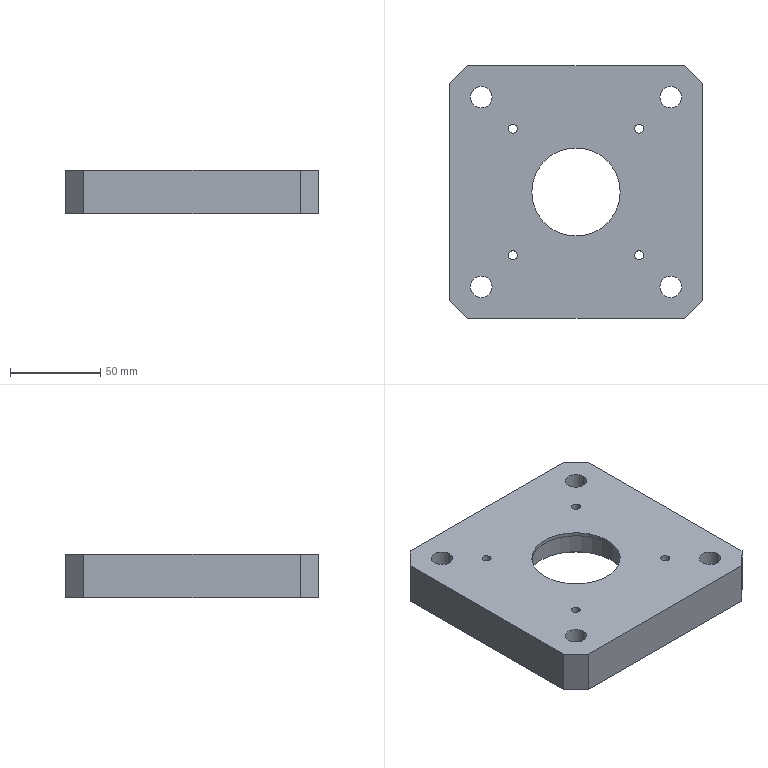Part | SolidWorks | features HoleWzd 3, ICE 3, Chamfer 1, Cut 1, Extrusion 1 | 1 solid | 46 faces | box 140 x 140 x 24 mm | volume 366967 mm3 | cylinder 30 | plane 16 | commonest cylinder face diameters 5 x8 12 x8 18 x8 49 x2 55 x2 80 x2
STEP:
#1=CARTESIAN_POINT('',(40.,0.,9.));
#2=VERTEX_POINT('',#1);
#3=CARTESIAN_POINT('',(-40.,0.,9.));
#4=VERTEX_POINT('',#3);
#5=CARTESIAN_POINT('',(0.,0.,9.));
#6=DIRECTION('',(0.,0.,-1.));
#7=DIRECTION('',(-1.,0.,0.));
#8=AXIS2_PLACEMENT_3D('',#5,#6,#7);
#9=CIRCLE('',#8,40.);
#10=EDGE_CURVE('',#2,#4,#9,.T.);
#11=ORIENTED_EDGE('',*,*,#10,.F.);
#12=CARTESIAN_POINT('',(40.,0.,0.));
#13=VERTEX_POINT('',#12);
#14=CARTESIAN_POINT('',(40.,0.,9.));
#15=DIRECTION('',(0.,0.,-1.));
#16=VECTOR('',#15,1000.);
#17=LINE('',#14,#16);
#18=EDGE_CURVE('',#2,#13,#17,.T.);
#19=ORIENTED_EDGE('',*,*,#18,.T.);
#20=CARTESIAN_POINT('',(-40.,0.,0.));
#21=VERTEX_POINT('',#20);
#22=CARTESIAN_POINT('',(0.,0.,0.));
#23=DIRECTION('',(0.,0.,-1.));
#24=DIRECTION('',(-1.,0.,0.));
#25=AXIS2_PLACEMENT_3D('',#22,#23,#24);
#26=CIRCLE('',#25,40.);
#27=EDGE_CURVE('',#13,#21,#26,.T.);
#28=ORIENTED_EDGE('',*,*,#27,.T.);
#29=CARTESIAN_POINT('',(-40.,0.,9.));
#30=DIRECTION('',(0.,0.,-1.));
#31=VECTOR('',#30,1000.);
#32=LINE('',#29,#31);
#33=EDGE_CURVE('',#4,#21,#32,.T.);
#34=ORIENTED_EDGE('',*,*,#33,.F.);
#35=EDGE_LOOP('',(#11,#19,#28,#34));
#36=FACE_OUTER_BOUND('',#35,.T.);
#37=CARTESIAN_POINT('',(0.,0.,9.));
#38=DIRECTION('',(0.,0.,-1.));
#39=DIRECTION('',(-1.,0.,0.));
#40=AXIS2_PLACEMENT_3D('',#37,#38,#39);
#41=CYLINDRICAL_SURFACE('',#40,40.);
#42=ADVANCED_FACE('',(#36),#41,.F.);
#43=CARTESIAN_POINT('',(37.5,35.,24.));
#44=VERTEX_POINT('',#43);
#45=CARTESIAN_POINT('',(32.5,35.,24.));
#46=VERTEX_POINT('',#45);
#47=CARTESIAN_POINT('',(35.,35.,24.));
#48=DIRECTION('',(0.,0.,-1.));
#49=DIRECTION('',(-1.,0.,0.));
#50=AXIS2_PLACEMENT_3D('',#47,#48,#49);
#51=CIRCLE('',#50,2.5);
#52=EDGE_CURVE('',#44,#46,#51,.T.);
#53=ORIENTED_EDGE('',*,*,#52,.F.);
#54=CARTESIAN_POINT('',(37.5,35.,0.));
#55=VERTEX_POINT('',#54);
#56=CARTESIAN_POINT('',(37.5,35.,0.));
#57=DIRECTION('',(0.,0.,-1.));
#58=VECTOR('',#57,1000.);
#59=LINE('',#56,#58);
#60=EDGE_CURVE('',#44,#55,#59,.T.);
#61=ORIENTED_EDGE('',*,*,#60,.T.);
#62=CARTESIAN_POINT('',(32.5,35.,0.));
#63=VERTEX_POINT('',#62);
#64=CARTESIAN_POINT('',(35.,35.,0.));
#65=DIRECTION('',(0.,0.,-1.));
#66=DIRECTION('',(-1.,0.,0.));
#67=AXIS2_PLACEMENT_3D('',#64,#65,#66);
#68=CIRCLE('',#67,2.5);
#69=EDGE_CURVE('',#55,#63,#68,.T.);
#70=ORIENTED_EDGE('',*,*,#69,.T.);
#71=CARTESIAN_POINT('',(32.5,35.,0.));
#72=DIRECTION('',(0.,0.,-1.));
#73=VECTOR('',#72,1000.);
#74=LINE('',#71,#73);
#75=EDGE_CURVE('',#46,#63,#74,.T.);
#76=ORIENTED_EDGE('',*,*,#75,.F.);
#77=EDGE_LOOP('',(#53,#61,#70,#76));
#78=FACE_OUTER_BOUND('',#77,.T.);
#79=CARTESIAN_POINT('',(35.,35.,0.));
#80=DIRECTION('',(0.,0.,-1.));
#81=DIRECTION('',(-1.,0.,0.));
#82=AXIS2_PLACEMENT_3D('',#79,#80,#81);
#83=CYLINDRICAL_SURFACE('',#82,2.5);
#84=ADVANCED_FACE('',(#78),#83,.F.);
#85=CARTESIAN_POINT('',(-32.5,35.,24.));
#86=VERTEX_POINT('',#85);
#87=CARTESIAN_POINT('',(-37.5,35.,24.));
#88=VERTEX_POINT('',#87);
#89=CARTESIAN_POINT('',(-35.,35.,24.));
#90=DIRECTION('',(0.,0.,-1.));
#91=DIRECTION('',(-1.,0.,0.));
#92=AXIS2_PLACEMENT_3D('',#89,#90,#91);
#93=CIRCLE('',#92,2.5);
#94=EDGE_CURVE('',#86,#88,#93,.T.);
#95=ORIENTED_EDGE('',*,*,#94,.F.);
#96=CARTESIAN_POINT('',(-32.5,35.,0.));
#97=VERTEX_POINT('',#96);
#98=CARTESIAN_POINT('',(-32.5,35.,0.));
#99=DIRECTION('',(0.,0.,-1.));
#100=VECTOR('',#99,1000.);
#101=LINE('',#98,#100);
#102=EDGE_CURVE('',#86,#97,#101,.T.);
#103=ORIENTED_EDGE('',*,*,#102,.T.);
#104=CARTESIAN_POINT('',(-37.5,35.,0.));
#105=VERTEX_POINT('',#104);
#106=CARTESIAN_POINT('',(-35.,35.,0.));
#107=DIRECTION('',(0.,0.,-1.));
#108=DIRECTION('',(-1.,0.,0.));
#109=AXIS2_PLACEMENT_3D('',#106,#107,#108);
#110=CIRCLE('',#109,2.5);
#111=EDGE_CURVE('',#97,#105,#110,.T.);
#112=ORIENTED_EDGE('',*,*,#111,.T.);
#113=CARTESIAN_POINT('',(-37.5,35.,0.));
#114=DIRECTION('',(0.,0.,-1.));
#115=VECTOR('',#114,1000.);
#116=LINE('',#113,#115);
#117=EDGE_CURVE('',#88,#105,#116,.T.);
#118=ORIENTED_EDGE('',*,*,#117,.F.);
#119=EDGE_LOOP('',(#95,#103,#112,#118));
#120=FACE_OUTER_BOUND('',#119,.T.);
#121=CARTESIAN_POINT('',(-35.,35.,0.));
#122=DIRECTION('',(0.,0.,-1.));
#123=DIRECTION('',(-1.,0.,0.));
#124=AXIS2_PLACEMENT_3D('',#121,#122,#123);
#125=CYLINDRICAL_SURFACE('',#124,2.5);
#126=ADVANCED_FACE('',(#120),#125,.F.);
#127=CARTESIAN_POINT('',(-32.5,-35.,24.));
#128=VERTEX_POINT('',#127);
#129=CARTESIAN_POINT('',(-37.5,-35.,24.));
#130=VERTEX_POINT('',#129);
#131=CARTESIAN_POINT('',(-35.,-35.,24.));
#132=DIRECTION('',(0.,0.,-1.));
#133=DIRECTION('',(-1.,0.,0.));
#134=AXIS2_PLACEMENT_3D('',#131,#132,#133);
#135=CIRCLE('',#134,2.5);
#136=EDGE_CURVE('',#128,#130,#135,.T.);
#137=ORIENTED_EDGE('',*,*,#136,.F.);
#138=CARTESIAN_POINT('',(-32.5,-35.,0.));
#139=VERTEX_POINT('',#138);
#140=CARTESIAN_POINT('',(-32.5,-35.,0.));
#141=DIRECTION('',(0.,0.,-1.));
#142=VECTOR('',#141,1000.);
#143=LINE('',#140,#142);
#144=EDGE_CURVE('',#128,#139,#143,.T.);
#145=ORIENTED_EDGE('',*,*,#144,.T.);
#146=CARTESIAN_POINT('',(-37.5,-35.,0.));
#147=VERTEX_POINT('',#146);
#148=CARTESIAN_POINT('',(-35.,-35.,0.));
#149=DIRECTION('',(0.,0.,-1.));
#150=DIRECTION('',(-1.,0.,0.));
#151=AXIS2_PLACEMENT_3D('',#148,#149,#150);
#152=CIRCLE('',#151,2.5);
#153=EDGE_CURVE('',#139,#147,#152,.T.);
#154=ORIENTED_EDGE('',*,*,#153,.T.);
#155=CARTESIAN_POINT('',(-37.5,-35.,0.));
#156=DIRECTION('',(0.,0.,-1.));
#157=VECTOR('',#156,1000.);
#158=LINE('',#155,#157);
#159=EDGE_CURVE('',#130,#147,#158,.T.);
#160=ORIENTED_EDGE('',*,*,#159,.F.);
#161=EDGE_LOOP('',(#137,#145,#154,#160));
#162=FACE_OUTER_BOUND('',#161,.T.);
#163=CARTESIAN_POINT('',(-35.,-35.,0.));
#164=DIRECTION('',(0.,0.,-1.));
#165=DIRECTION('',(-1.,0.,0.));
#166=AXIS2_PLACEMENT_3D('',#163,#164,#165);
#167=CYLINDRICAL_SURFACE('',#166,2.5);
#168=ADVANCED_FACE('',(#162),#167,.F.);
#169=CARTESIAN_POINT('',(37.5,-35.,24.));
#170=VERTEX_POINT('',#169);
#171=CARTESIAN_POINT('',(32.5,-35.,24.));
#172=VERTEX_POINT('',#171);
#173=CARTESIAN_POINT('',(35.,-35.,24.));
#174=DIRECTION('',(0.,0.,-1.));
#175=DIRECTION('',(-1.,0.,0.));
#176=AXIS2_PLACEMENT_3D('',#173,#174,#175);
#177=CIRCLE('',#176,2.5);
#178=EDGE_CURVE('',#170,#172,#177,.T.);
#179=ORIENTED_EDGE('',*,*,#178,.F.);
#180=CARTESIAN_POINT('',(37.5,-35.,0.));
#181=VERTEX_POINT('',#180);
#182=CARTESIAN_POINT('',(37.5,-35.,0.));
#183=DIRECTION('',(0.,0.,-1.));
#184=VECTOR('',#183,1000.);
#185=LINE('',#182,#184);
#186=EDGE_CURVE('',#170,#181,#185,.T.);
#187=ORIENTED_EDGE('',*,*,#186,.T.);
#188=CARTESIAN_POINT('',(32.5,-35.,0.));
#189=VERTEX_POINT('',#188);
#190=CARTESIAN_POINT('',(35.,-35.,0.));
#191=DIRECTION('',(0.,0.,-1.));
#192=DIRECTION('',(-1.,0.,0.));
#193=AXIS2_PLACEMENT_3D('',#190,#191,#192);
#194=CIRCLE('',#193,2.5);
#195=EDGE_CURVE('',#181,#189,#194,.T.);
#196=ORIENTED_EDGE('',*,*,#195,.T.);
#197=CARTESIAN_POINT('',(32.5,-35.,0.));
#198=DIRECTION('',(0.,0.,-1.));
#199=VECTOR('',#198,1000.);
#200=LINE('',#197,#199);
#201=EDGE_CURVE('',#172,#189,#200,.T.);
#202=ORIENTED_EDGE('',*,*,#201,.F.);
#203=EDGE_LOOP('',(#179,#187,#196,#202));
#204=FACE_OUTER_BOUND('',#203,.T.);
#205=CARTESIAN_POINT('',(35.,-35.,0.));
#206=DIRECTION('',(0.,0.,-1.));
#207=DIRECTION('',(-1.,0.,0.));
#208=AXIS2_PLACEMENT_3D('',#205,#206,#207);
#209=CYLINDRICAL_SURFACE('',#208,2.5);
#210=ADVANCED_FACE('',(#204),#209,.F.);
#211=CARTESIAN_POINT('',(61.5,52.5,10.6));
#212=VERTEX_POINT('',#211);
#213=CARTESIAN_POINT('',(43.5,52.5,10.6));
#214=VERTEX_POINT('',#213);
#215=CARTESIAN_POINT('',(52.5,52.5,10.6));
#216=DIRECTION('',(0.,0.,-1.));
#217=DIRECTION('',(-1.,0.,0.));
#218=AXIS2_PLACEMENT_3D('',#215,#216,#217);
#219=CIRCLE('',#218,9.);
#220=EDGE_CURVE('',#212,#214,#219,.T.);
#221=ORIENTED_EDGE('',*,*,#220,.F.);
#222=CARTESIAN_POINT('',(61.5,52.5,0.));
#223=VERTEX_POINT('',#222);
#224=CARTESIAN_POINT('',(61.5,52.5,0.));
#225=DIRECTION('',(0.,0.,-1.));
#226=VECTOR('',#225,1000.);
#227=LINE('',#224,#226);
#228=EDGE_CURVE('',#212,#223,#227,.T.);
#229=ORIENTED_EDGE('',*,*,#228,.T.);
#230=CARTESIAN_POINT('',(43.5,52.5,0.));
#231=VERTEX_POINT('',#230);
#232=CARTESIAN_POINT('',(52.5,52.5,0.));
#233=DIRECTION('',(0.,0.,-1.));
#234=DIRECTION('',(-1.,0.,0.));
#235=AXIS2_PLACEMENT_3D('',#232,#233,#234);
#236=CIRCLE('',#235,9.);
#237=EDGE_CURVE('',#223,#231,#236,.T.);
#238=ORIENTED_EDGE('',*,*,#237,.T.);
#239=CARTESIAN_POINT('',(43.5,52.5,0.));
#240=DIRECTION('',(0.,0.,-1.));
#241=VECTOR('',#240,1000.);
#242=LINE('',#239,#241);
#243=EDGE_CURVE('',#214,#231,#242,.T.);
#244=ORIENTED_EDGE('',*,*,#243,.F.);
#245=EDGE_LOOP('',(#221,#229,#238,#244));
#246=FACE_OUTER_BOUND('',#245,.T.);
#247=CARTESIAN_POINT('',(52.5,52.5,0.));
#248=DIRECTION('',(0.,0.,-1.));
#249=DIRECTION('',(-1.,0.,0.));
#250=AXIS2_PLACEMENT_3D('',#247,#248,#249);
#251=CYLINDRICAL_SURFACE('',#250,9.);
#252=ADVANCED_FACE('',(#246),#251,.F.);
#253=CARTESIAN_POINT('',(58.5,52.5,24.));
#254=VERTEX_POINT('',#253);
#255=CARTESIAN_POINT('',(46.5,52.5,24.));
#256=VERTEX_POINT('',#255);
#257=CARTESIAN_POINT('',(52.5,52.5,24.));
#258=DIRECTION('',(0.,0.,-1.));
#259=DIRECTION('',(-1.,0.,0.));
#260=AXIS2_PLACEMENT_3D('',#257,#258,#259);
#261=CIRCLE('',#260,6.);
#262=EDGE_CURVE('',#254,#256,#261,.T.);
#263=ORIENTED_EDGE('',*,*,#262,.F.);
#264=CARTESIAN_POINT('',(58.5,52.5,10.6));
#265=VERTEX_POINT('',#264);
#266=CARTESIAN_POINT('',(58.5,52.5,0.));
#267=DIRECTION('',(0.,0.,-1.));
#268=VECTOR('',#267,1000.);
#269=LINE('',#266,#268);
#270=EDGE_CURVE('',#254,#265,#269,.T.);
#271=ORIENTED_EDGE('',*,*,#270,.T.);
#272=CARTESIAN_POINT('',(46.5,52.5,10.6));
#273=VERTEX_POINT('',#272);
#274=CARTESIAN_POINT('',(52.5,52.5,10.6));
#275=DIRECTION('',(0.,0.,-1.));
#276=DIRECTION('',(-1.,0.,0.));
#277=AXIS2_PLACEMENT_3D('',#274,#275,#276);
#278=CIRCLE('',#277,6.);
#279=EDGE_CURVE('',#265,#273,#278,.T.);
#280=ORIENTED_EDGE('',*,*,#279,.T.);
#281=CARTESIAN_POINT('',(46.5,52.5,0.));
#282=DIRECTION('',(0.,0.,-1.));
#283=VECTOR('',#282,1000.);
#284=LINE('',#281,#283);
#285=EDGE_CURVE('',#256,#273,#284,.T.);
#286=ORIENTED_EDGE('',*,*,#285,.F.);
#287=EDGE_LOOP('',(#263,#271,#280,#286));
#288=FACE_OUTER_BOUND('',#287,.T.);
#289=CARTESIAN_POINT('',(52.5,52.5,0.));
#290=DIRECTION('',(0.,0.,-1.));
#291=DIRECTION('',(-1.,0.,0.));
#292=AXIS2_PLACEMENT_3D('',#289,#290,#291);
#293=CYLINDRICAL_SURFACE('',#292,6.);
#294=ADVANCED_FACE('',(#288),#293,.F.);
#295=CARTESIAN_POINT('',(-43.5,52.5,10.6));
#296=VERTEX_POINT('',#295);
#297=CARTESIAN_POINT('',(-61.5,52.5,10.6));
#298=VERTEX_POINT('',#297);
#299=CARTESIAN_POINT('',(-52.5,52.5,10.6));
#300=DIRECTION('',(0.,0.,-1.));
#301=DIRECTION('',(-1.,0.,0.));
#302=AXIS2_PLACEMENT_3D('',#299,#300,#301);
#303=CIRCLE('',#302,9.);
#304=EDGE_CURVE('',#296,#298,#303,.T.);
#305=ORIENTED_EDGE('',*,*,#304,.F.);
#306=CARTESIAN_POINT('',(-43.5,52.5,0.));
#307=VERTEX_POINT('',#306);
#308=CARTESIAN_POINT('',(-43.5,52.5,0.));
#309=DIRECTION('',(0.,0.,-1.));
#310=VECTOR('',#309,1000.);
#311=LINE('',#308,#310);
#312=EDGE_CURVE('',#296,#307,#311,.T.);
#313=ORIENTED_EDGE('',*,*,#312,.T.);
#314=CARTESIAN_POINT('',(-61.5,52.5,0.));
#315=VERTEX_POINT('',#314);
#316=CARTESIAN_POINT('',(-52.5,52.5,0.));
#317=DIRECTION('',(0.,0.,-1.));
#318=DIRECTION('',(-1.,0.,0.));
#319=AXIS2_PLACEMENT_3D('',#316,#317,#318);
#320=CIRCLE('',#319,9.);
#321=EDGE_CURVE('',#307,#315,#320,.T.);
#322=ORIENTED_EDGE('',*,*,#321,.T.);
#323=CARTESIAN_POINT('',(-61.5,52.5,0.));
#324=DIRECTION('',(0.,0.,-1.));
#325=VECTOR('',#324,1000.);
#326=LINE('',#323,#325);
#327=EDGE_CURVE('',#298,#315,#326,.T.);
#328=ORIENTED_EDGE('',*,*,#327,.F.);
#329=EDGE_LOOP('',(#305,#313,#322,#328));
#330=FACE_OUTER_BOUND('',#329,.T.);
#331=CARTESIAN_POINT('',(-52.5,52.5,0.));
#332=DIRECTION('',(0.,0.,-1.));
#333=DIRECTION('',(-1.,0.,0.));
#334=AXIS2_PLACEMENT_3D('',#331,#332,#333);
#335=CYLINDRICAL_SURFACE('',#334,9.);
#336=ADVANCED_FACE('',(#330),#335,.F.);
#337=CARTESIAN_POINT('',(-46.5,52.5,24.));
#338=VERTEX_POINT('',#337);
#339=CARTESIAN_POINT('',(-58.5,52.5,24.));
#340=VERTEX_POINT('',#339);
#341=CARTESIAN_POINT('',(-52.5,52.5,24.));
#342=DIRECTION('',(0.,0.,-1.));
#343=DIRECTION('',(-1.,0.,0.));
#344=AXIS2_PLACEMENT_3D('',#341,#342,#343);
#345=CIRCLE('',#344,6.);
#346=EDGE_CURVE('',#338,#340,#345,.T.);
#347=ORIENTED_EDGE('',*,*,#346,.F.);
#348=CARTESIAN_POINT('',(-46.5,52.5,10.6));
#349=VERTEX_POINT('',#348);
#350=CARTESIAN_POINT('',(-46.5,52.5,0.));
#351=DIRECTION('',(0.,0.,-1.));
#352=VECTOR('',#351,1000.);
#353=LINE('',#350,#352);
#354=EDGE_CURVE('',#338,#349,#353,.T.);
#355=ORIENTED_EDGE('',*,*,#354,.T.);
#356=CARTESIAN_POINT('',(-58.5,52.5,10.6));
#357=VERTEX_POINT('',#356);
#358=CARTESIAN_POINT('',(-52.5,52.5,10.6));
#359=DIRECTION('',(0.,0.,-1.));
#360=DIRECTION('',(-1.,0.,0.));
#361=AXIS2_PLACEMENT_3D('',#358,#359,#360);
#362=CIRCLE('',#361,6.);
#363=EDGE_CURVE('',#349,#357,#362,.T.);
#364=ORIENTED_EDGE('',*,*,#363,.T.);
#365=CARTESIAN_POINT('',(-58.5,52.5,0.));
#366=DIRECTION('',(0.,0.,-1.));
#367=VECTOR('',#366,1000.);
#368=LINE('',#365,#367);
#369=EDGE_CURVE('',#340,#357,#368,.T.);
#370=ORIENTED_EDGE('',*,*,#369,.F.);
#371=EDGE_LOOP('',(#347,#355,#364,#370));
#372=FACE_OUTER_BOUND('',#371,.T.);
#373=CARTESIAN_POINT('',(-52.5,52.5,0.));
#374=DIRECTION('',(0.,0.,-1.));
#375=DIRECTION('',(-1.,0.,0.));
#376=AXIS2_PLACEMENT_3D('',#373,#374,#375);
#377=CYLINDRICAL_SURFACE('',#376,6.);
#378=ADVANCED_FACE('',(#372),#377,.F.);
#379=CARTESIAN_POINT('',(-43.5,-52.5,10.6));
#380=VERTEX_POINT('',#379);
#381=CARTESIAN_POINT('',(-61.5,-52.5,10.6));
#382=VERTEX_POINT('',#381);
#383=CARTESIAN_POINT('',(-52.5,-52.5,10.6));
#384=DIRECTION('',(0.,0.,-1.));
#385=DIRECTION('',(-1.,0.,0.));
#386=AXIS2_PLACEMENT_3D('',#383,#384,#385);
#387=CIRCLE('',#386,9.);
#388=EDGE_CURVE('',#380,#382,#387,.T.);
#389=ORIENTED_EDGE('',*,*,#388,.F.);
#390=CARTESIAN_POINT('',(-43.5,-52.5,0.));
#391=VERTEX_POINT('',#390);
#392=CARTESIAN_POINT('',(-43.5,-52.5,0.));
#393=DIRECTION('',(0.,0.,-1.));
#394=VECTOR('',#393,1000.);
#395=LINE('',#392,#394);
#396=EDGE_CURVE('',#380,#391,#395,.T.);
#397=ORIENTED_EDGE('',*,*,#396,.T.);
#398=CARTESIAN_POINT('',(-61.5,-52.5,0.));
#399=VERTEX_POINT('',#398);
#400=CARTESIAN_POINT('',(-52.5,-52.5,0.));
#401=DIRECTION('',(0.,0.,-1.));
#402=DIRECTION('',(-1.,0.,0.));
#403=AXIS2_PLACEMENT_3D('',#400,#401,#402);
#404=CIRCLE('',#403,9.);
#405=EDGE_CURVE('',#391,#399,#404,.T.);
#406=ORIENTED_EDGE('',*,*,#405,.T.);
#407=CARTESIAN_POINT('',(-61.5,-52.5,0.));
#408=DIRECTION('',(0.,0.,-1.));
#409=VECTOR('',#408,1000.);
#410=LINE('',#407,#409);
#411=EDGE_CURVE('',#382,#399,#410,.T.);
#412=ORIENTED_EDGE('',*,*,#411,.F.);
#413=EDGE_LOOP('',(#389,#397,#406,#412));
#414=FACE_OUTER_BOUND('',#413,.T.);
#415=CARTESIAN_POINT('',(-52.5,-52.5,0.));
#416=DIRECTION('',(0.,0.,-1.));
#417=DIRECTION('',(-1.,0.,0.));
#418=AXIS2_PLACEMENT_3D('',#415,#416,#417);
#419=CYLINDRICAL_SURFACE('',#418,9.);
#420=ADVANCED_FACE('',(#414),#419,.F.);
#421=CARTESIAN_POINT('',(-46.5,-52.5,24.));
#422=VERTEX_POINT('',#421);
#423=CARTESIAN_POINT('',(-58.5,-52.5,24.));
#424=VERTEX_POINT('',#423);
#425=CARTESIAN_POINT('',(-52.5,-52.5,24.));
#426=DIRECTION('',(0.,0.,-1.));
#427=DIRECTION('',(-1.,0.,0.));
#428=AXIS2_PLACEMENT_3D('',#425,#426,#427);
#429=CIRCLE('',#428,6.);
#430=EDGE_CURVE('',#422,#424,#429,.T.);
#431=ORIENTED_EDGE('',*,*,#430,.F.);
#432=CARTESIAN_POINT('',(-46.5,-52.5,10.6));
#433=VERTEX_POINT('',#432);
#434=CARTESIAN_POINT('',(-46.5,-52.5,0.));
#435=DIRECTION('',(0.,0.,-1.));
#436=VECTOR('',#435,1000.);
#437=LINE('',#434,#436);
#438=EDGE_CURVE('',#422,#433,#437,.T.);
#439=ORIENTED_EDGE('',*,*,#438,.T.);
#440=CARTESIAN_POINT('',(-58.5,-52.5,10.6));
#441=VERTEX_POINT('',#440);
#442=CARTESIAN_POINT('',(-52.5,-52.5,10.6));
#443=DIRECTION('',(0.,0.,-1.));
#444=DIRECTION('',(-1.,0.,0.));
#445=AXIS2_PLACEMENT_3D('',#442,#443,#444);
#446=CIRCLE('',#445,6.);
#447=EDGE_CURVE('',#433,#441,#446,.T.);
#448=ORIENTED_EDGE('',*,*,#447,.T.);
#449=CARTESIAN_POINT('',(-58.5,-52.5,0.));
#450=DIRECTION('',(0.,0.,-1.));
#451=VECTOR('',#450,1000.);
#452=LINE('',#449,#451);
#453=EDGE_CURVE('',#424,#441,#452,.T.);
#454=ORIENTED_EDGE('',*,*,#453,.F.);
#455=EDGE_LOOP('',(#431,#439,#448,#454));
#456=FACE_OUTER_BOUND('',#455,.T.);
#457=CARTESIAN_POINT('',(-52.5,-52.5,0.));
#458=DIRECTION('',(0.,0.,-1.));
#459=DIRECTION('',(-1.,0.,0.));
#460=AXIS2_PLACEMENT_3D('',#457,#458,#459);
#461=CYLINDRICAL_SURFACE('',#460,6.);
#462=ADVANCED_FACE('',(#456),#461,.F.);
#463=CARTESIAN_POINT('',(61.5,-52.5,10.6));
#464=VERTEX_POINT('',#463);
#465=CARTESIAN_POINT('',(43.5,-52.5,10.6));
#466=VERTEX_POINT('',#465);
#467=CARTESIAN_POINT('',(52.5,-52.5,10.6));
#468=DIRECTION('',(0.,0.,-1.));
#469=DIRECTION('',(-1.,0.,0.));
#470=AXIS2_PLACEMENT_3D('',#467,#468,#469);
#471=CIRCLE('',#470,9.);
#472=EDGE_CURVE('',#464,#466,#471,.T.);
#473=ORIENTED_EDGE('',*,*,#472,.F.);
#474=CARTESIAN_POINT('',(61.5,-52.5,0.));
#475=VERTEX_POINT('',#474);
#476=CARTESIAN_POINT('',(61.5,-52.5,0.));
#477=DIRECTION('',(0.,0.,-1.));
#478=VECTOR('',#477,1000.);
#479=LINE('',#476,#478);
#480=EDGE_CURVE('',#464,#475,#479,.T.);
#481=ORIENTED_EDGE('',*,*,#480,.T.);
#482=CARTESIAN_POINT('',(43.5,-52.5,0.));
#483=VERTEX_POINT('',#482);
#484=CARTESIAN_POINT('',(52.5,-52.5,0.));
#485=DIRECTION('',(0.,0.,-1.));
#486=DIRECTION('',(-1.,0.,0.));
#487=AXIS2_PLACEMENT_3D('',#484,#485,#486);
#488=CIRCLE('',#487,9.);
#489=EDGE_CURVE('',#475,#483,#488,.T.);
#490=ORIENTED_EDGE('',*,*,#489,.T.);
#491=CARTESIAN_POINT('',(43.5,-52.5,0.));
#492=DIRECTION('',(0.,0.,-1.));
#493=VECTOR('',#492,1000.);
#494=LINE('',#491,#493);
#495=EDGE_CURVE('',#466,#483,#494,.T.);
#496=ORIENTED_EDGE('',*,*,#495,.F.);
#497=EDGE_LOOP('',(#473,#481,#490,#496));
#498=FACE_OUTER_BOUND('',#497,.T.);
#499=CARTESIAN_POINT('',(52.5,-52.5,0.));
#500=DIRECTION('',(0.,0.,-1.));
#501=DIRECTION('',(-1.,0.,0.));
#502=AXIS2_PLACEMENT_3D('',#499,#500,#501);
#503=CYLINDRICAL_SURFACE('',#502,9.);
#504=ADVANCED_FACE('',(#498),#503,.F.);
#505=CARTESIAN_POINT('',(58.5,-52.5,24.));
#506=VERTEX_POINT('',#505);
#507=CARTESIAN_POINT('',(46.5,-52.5,24.));
#508=VERTEX_POINT('',#507);
#509=CARTESIAN_POINT('',(52.5,-52.5,24.));
#510=DIRECTION('',(0.,0.,-1.));
#511=DIRECTION('',(-1.,0.,0.));
#512=AXIS2_PLACEMENT_3D('',#509,#510,#511);
#513=CIRCLE('',#512,6.);
#514=EDGE_CURVE('',#506,#508,#513,.T.);
#515=ORIENTED_EDGE('',*,*,#514,.F.);
#516=CARTESIAN_POINT('',(58.5,-52.5,10.6));
#517=VERTEX_POINT('',#516);
#518=CARTESIAN_POINT('',(58.5,-52.5,0.));
#519=DIRECTION('',(0.,0.,-1.));
#520=VECTOR('',#519,1000.);
#521=LINE('',#518,#520);
#522=EDGE_CURVE('',#506,#517,#521,.T.);
#523=ORIENTED_EDGE('',*,*,#522,.T.);
#524=CARTESIAN_POINT('',(46.5,-52.5,10.6));
#525=VERTEX_POINT('',#524);
#526=CARTESIAN_POINT('',(52.5,-52.5,10.6));
#527=DIRECTION('',(0.,0.,-1.));
#528=DIRECTION('',(-1.,0.,0.));
#529=AXIS2_PLACEMENT_3D('',#526,#527,#528);
#530=CIRCLE('',#529,6.);
#531=EDGE_CURVE('',#517,#525,#530,.T.);
#532=ORIENTED_EDGE('',*,*,#531,.T.);
#533=CARTESIAN_POINT('',(46.5,-52.5,0.));
#534=DIRECTION('',(0.,0.,-1.));
#535=VECTOR('',#534,1000.);
#536=LINE('',#533,#535);
#537=EDGE_CURVE('',#508,#525,#536,.T.);
#538=ORIENTED_EDGE('',*,*,#537,.F.);
#539=EDGE_LOOP('',(#515,#523,#532,#538));
#540=FACE_OUTER_BOUND('',#539,.T.);
#541=CARTESIAN_POINT('',(52.5,-52.5,0.));
#542=DIRECTION('',(0.,0.,-1.));
#543=DIRECTION('',(-1.,0.,0.));
#544=AXIS2_PLACEMENT_3D('',#541,#542,#543);
#545=CYLINDRICAL_SURFACE('',#544,6.);
#546=ADVANCED_FACE('',(#540),#545,.F.);
#547=CARTESIAN_POINT('',(24.5,0.,24.));
#548=VERTEX_POINT('',#547);
#549=CARTESIAN_POINT('',(-24.5,0.,24.));
#550=VERTEX_POINT('',#549);
#551=CARTESIAN_POINT('',(0.,0.,24.));
#552=DIRECTION('',(0.,0.,-1.));
#553=DIRECTION('',(-1.,0.,0.));
#554=AXIS2_PLACEMENT_3D('',#551,#552,#553);
#555=CIRCLE('',#554,24.5);
#556=EDGE_CURVE('',#548,#550,#555,.T.);
#557=ORIENTED_EDGE('',*,*,#556,.F.);
#558=CARTESIAN_POINT('',(24.5,0.,22.));
#559=VERTEX_POINT('',#558);
#560=CARTESIAN_POINT('',(24.5,0.,24.));
#561=DIRECTION('',(0.,0.,-1.));
#562=VECTOR('',#561,1000.);
#563=LINE('',#560,#562);
#564=EDGE_CURVE('',#548,#559,#563,.T.);
#565=ORIENTED_EDGE('',*,*,#564,.T.);
#566=CARTESIAN_POINT('',(-24.5,0.,22.));
#567=VERTEX_POINT('',#566);
#568=CARTESIAN_POINT('',(0.,0.,22.));
#569=DIRECTION('',(0.,0.,-1.));
#570=DIRECTION('',(-1.,0.,0.));
#571=AXIS2_PLACEMENT_3D('',#568,#569,#570);
#572=CIRCLE('',#571,24.5);
#573=EDGE_CURVE('',#559,#567,#572,.T.);
#574=ORIENTED_EDGE('',*,*,#573,.T.);
#575=CARTESIAN_POINT('',(-24.5,0.,24.));
#576=DIRECTION('',(0.,0.,-1.));
#577=VECTOR('',#576,1000.);
#578=LINE('',#575,#577);
#579=EDGE_CURVE('',#550,#567,#578,.T.);
#580=ORIENTED_EDGE('',*,*,#579,.F.);
#581=EDGE_LOOP('',(#557,#565,#574,#580));
#582=FACE_OUTER_BOUND('',#581,.T.);
#583=CARTESIAN_POINT('',(0.,0.,24.));
#584=DIRECTION('',(0.,0.,-1.));
#585=DIRECTION('',(-1.,0.,0.));
#586=AXIS2_PLACEMENT_3D('',#583,#584,#585);
#587=CYLINDRICAL_SURFACE('',#586,24.5);
#588=ADVANCED_FACE('',(#582),#587,.F.);
#589=CARTESIAN_POINT('',(-27.5,0.,22.));
#590=VERTEX_POINT('',#589);
#591=CARTESIAN_POINT('',(27.5,0.,22.));
#592=VERTEX_POINT('',#591);
#593=CARTESIAN_POINT('',(0.,0.,22.));
#594=DIRECTION('',(0.,0.,1.));
#595=DIRECTION('',(-1.,0.,0.));
#596=AXIS2_PLACEMENT_3D('',#593,#594,#595);
#597=CIRCLE('',#596,27.5);
#598=EDGE_CURVE('',#590,#592,#597,.T.);
#599=ORIENTED_EDGE('',*,*,#598,.T.);
#600=CARTESIAN_POINT('',(27.5,0.,9.));
#601=VERTEX_POINT('',#600);
#602=CARTESIAN_POINT('',(27.5,0.,101.782));
#603=DIRECTION('',(0.,0.,-1.));
#604=VECTOR('',#603,1000.);
#605=LINE('',#602,#604);
#606=EDGE_CURVE('',#592,#601,#605,.T.);
#607=ORIENTED_EDGE('',*,*,#606,.T.);
#608=CARTESIAN_POINT('',(-27.5,0.,9.));
#609=VERTEX_POINT('',#608);
#610=CARTESIAN_POINT('',(0.,0.,9.));
#611=DIRECTION('',(0.,0.,1.));
#612=DIRECTION('',(-1.,0.,0.));
#613=AXIS2_PLACEMENT_3D('',#610,#611,#612);
#614=CIRCLE('',#613,27.5);
#615=EDGE_CURVE('',#609,#601,#614,.T.);
#616=ORIENTED_EDGE('',*,*,#615,.F.);
#617=CARTESIAN_POINT('',(-27.5,0.,101.782));
#618=DIRECTION('',(0.,0.,-1.));
#619=VECTOR('',#618,1000.);
#620=LINE('',#617,#619);
#621=EDGE_CURVE('',#590,#609,#620,.T.);
#622=ORIENTED_EDGE('',*,*,#621,.F.);
#623=EDGE_LOOP('',(#599,#607,#616,#622));
#624=FACE_OUTER_BOUND('',#623,.T.);
#625=CARTESIAN_POINT('',(0.,0.,101.782));
#626=DIRECTION('',(0.,0.,-1.));
#627=DIRECTION('',(-1.,0.,0.));
#628=AXIS2_PLACEMENT_3D('',#625,#626,#627);
#629=CYLINDRICAL_SURFACE('',#628,27.5);
#630=ADVANCED_FACE('',(#624),#629,.F.);
#631=ORIENTED_EDGE('',*,*,#606,.F.);
#632=CARTESIAN_POINT('',(0.,0.,22.));
#633=DIRECTION('',(0.,0.,1.));
#634=DIRECTION('',(-1.,0.,0.));
#635=AXIS2_PLACEMENT_3D('',#632,#633,#634);
#636=CIRCLE('',#635,27.5);
#637=EDGE_CURVE('',#592,#590,#636,.T.);
#638=ORIENTED_EDGE('',*,*,#637,.T.);
#639=ORIENTED_EDGE('',*,*,#621,.T.);
#640=CARTESIAN_POINT('',(0.,0.,9.));
#641=DIRECTION('',(0.,0.,1.));
#642=DIRECTION('',(-1.,0.,0.));
#643=AXIS2_PLACEMENT_3D('',#640,#641,#642);
#644=CIRCLE('',#643,27.5);
#645=EDGE_CURVE('',#601,#609,#644,.T.);
#646=ORIENTED_EDGE('',*,*,#645,.F.);
#647=EDGE_LOOP('',(#631,#638,#639,#646));
#648=FACE_OUTER_BOUND('',#647,.T.);
#649=CARTESIAN_POINT('',(0.,0.,101.782));
#650=DIRECTION('',(0.,0.,-1.));
#651=DIRECTION('',(-1.,0.,0.));
#652=AXIS2_PLACEMENT_3D('',#649,#650,#651);
#653=CYLINDRICAL_SURFACE('',#652,27.5);
#654=ADVANCED_FACE('',(#648),#653,.F.);
#655=CARTESIAN_POINT('',(70.,-60.,24.));
#656=VERTEX_POINT('',#655);
#657=CARTESIAN_POINT('',(70.,60.,24.));
#658=VERTEX_POINT('',#657);
#659=CARTESIAN_POINT('',(70.,-70.,24.));
#660=DIRECTION('',(0.,1.,0.));
#661=VECTOR('',#660,1000.);
#662=LINE('',#659,#661);
#663=EDGE_CURVE('',#656,#658,#662,.T.);
#664=ORIENTED_EDGE('',*,*,#663,.F.);
#665=CARTESIAN_POINT('',(70.,-60.,0.));
#666=VERTEX_POINT('',#665);
#667=CARTESIAN_POINT('',(70.,-60.,24.));
#668=DIRECTION('',(0.,0.,-1.));
#669=VECTOR('',#668,1000.);
#670=LINE('',#667,#669);
#671=EDGE_CURVE('',#656,#666,#670,.T.);
#672=ORIENTED_EDGE('',*,*,#671,.T.);
#673=CARTESIAN_POINT('',(70.,60.,0.));
#674=VERTEX_POINT('',#673);
#675=CARTESIAN_POINT('',(70.,-70.,0.));
#676=DIRECTION('',(0.,1.,0.));
#677=VECTOR('',#676,1000.);
#678=LINE('',#675,#677);
#679=EDGE_CURVE('',#666,#674,#678,.T.);
#680=ORIENTED_EDGE('',*,*,#679,.T.);
#681=CARTESIAN_POINT('',(70.,60.,24.));
#682=DIRECTION('',(0.,0.,1.));
#683=VECTOR('',#682,1000.);
#684=LINE('',#681,#683);
#685=EDGE_CURVE('',#674,#658,#684,.T.);
#686=ORIENTED_EDGE('',*,*,#685,.T.);
#687=EDGE_LOOP('',(#664,#672,#680,#686));
#688=FACE_OUTER_BOUND('',#687,.T.);
#689=CARTESIAN_POINT('',(70.,-70.,24.));
#690=DIRECTION('',(-1.,0.,0.));
#691=DIRECTION('',(0.,0.,1.));
#692=AXIS2_PLACEMENT_3D('',#689,#690,#691);
#693=PLANE('',#692);
#694=ADVANCED_FACE('',(#688),#693,.F.);
#695=CARTESIAN_POINT('',(60.,70.,0.));
#696=VERTEX_POINT('',#695);
#697=CARTESIAN_POINT('',(-60.,70.,0.));
#698=VERTEX_POINT('',#697);
#699=CARTESIAN_POINT('',(-70.,70.,0.));
#700=DIRECTION('',(-1.,0.,0.));
#701=VECTOR('',#700,1000.);
#702=LINE('',#699,#701);
#703=EDGE_CURVE('',#696,#698,#702,.T.);
#704=ORIENTED_EDGE('',*,*,#703,.T.);
#705=CARTESIAN_POINT('',(-60.,70.,24.));
#706=VERTEX_POINT('',#705);
#707=CARTESIAN_POINT('',(-60.,70.,24.));
#708=DIRECTION('',(0.,0.,1.));
#709=VECTOR('',#708,1000.);
#710=LINE('',#707,#709);
#711=EDGE_CURVE('',#698,#706,#710,.T.);
#712=ORIENTED_EDGE('',*,*,#711,.T.);
#713=CARTESIAN_POINT('',(60.,70.,24.));
#714=VERTEX_POINT('',#713);
#715=CARTESIAN_POINT('',(-70.,70.,24.));
#716=DIRECTION('',(-1.,0.,0.));
#717=VECTOR('',#716,1000.);
#718=LINE('',#715,#717);
#719=EDGE_CURVE('',#714,#706,#718,.T.);
#720=ORIENTED_EDGE('',*,*,#719,.F.);
#721=CARTESIAN_POINT('',(60.,70.,24.));
#722=DIRECTION('',(0.,0.,-1.));
#723=VECTOR('',#722,1000.);
#724=LINE('',#721,#723);
#725=EDGE_CURVE('',#714,#696,#724,.T.);
#726=ORIENTED_EDGE('',*,*,#725,.T.);
#727=EDGE_LOOP('',(#704,#712,#720,#726));
#728=FACE_OUTER_BOUND('',#727,.T.);
#729=CARTESIAN_POINT('',(-70.,70.,24.));
#730=DIRECTION('',(0.,-1.,0.));
#731=DIRECTION('',(0.,0.,-1.));
#732=AXIS2_PLACEMENT_3D('',#729,#730,#731);
#733=PLANE('',#732);
#734=ADVANCED_FACE('',(#728),#733,.F.);
#735=CARTESIAN_POINT('',(-70.,60.,0.));
#736=VERTEX_POINT('',#735);
#737=CARTESIAN_POINT('',(-70.,-60.,0.));
#738=VERTEX_POINT('',#737);
#739=CARTESIAN_POINT('',(-70.,-70.,0.));
#740=DIRECTION('',(0.,-1.,0.));
#741=VECTOR('',#740,1000.);
#742=LINE('',#739,#741);
#743=EDGE_CURVE('',#736,#738,#742,.T.);
#744=ORIENTED_EDGE('',*,*,#743,.T.);
#745=CARTESIAN_POINT('',(-70.,-60.,24.));
#746=VERTEX_POINT('',#745);
#747=CARTESIAN_POINT('',(-70.,-60.,24.));
#748=DIRECTION('',(0.,0.,1.));
#749=VECTOR('',#748,1000.);
#750=LINE('',#747,#749);
#751=EDGE_CURVE('',#738,#746,#750,.T.);
#752=ORIENTED_EDGE('',*,*,#751,.T.);
#753=CARTESIAN_POINT('',(-70.,60.,24.));
#754=VERTEX_POINT('',#753);
#755=CARTESIAN_POINT('',(-70.,-70.,24.));
#756=DIRECTION('',(0.,-1.,0.));
#757=VECTOR('',#756,1000.);
#758=LINE('',#755,#757);
#759=EDGE_CURVE('',#754,#746,#758,.T.);
#760=ORIENTED_EDGE('',*,*,#759,.F.);
#761=CARTESIAN_POINT('',(-70.,60.,24.));
#762=DIRECTION('',(0.,0.,-1.));
#763=VECTOR('',#762,1000.);
#764=LINE('',#761,#763);
#765=EDGE_CURVE('',#754,#736,#764,.T.);
#766=ORIENTED_EDGE('',*,*,#765,.T.);
#767=EDGE_LOOP('',(#744,#752,#760,#766));
#768=FACE_OUTER_BOUND('',#767,.T.);
#769=CARTESIAN_POINT('',(-70.,-70.,24.));
#770=DIRECTION('',(1.,0.,0.));
#771=DIRECTION('',(0.,0.,-1.));
#772=AXIS2_PLACEMENT_3D('',#769,#770,#771);
#773=PLANE('',#772);
#774=ADVANCED_FACE('',(#768),#773,.F.);
#775=CARTESIAN_POINT('',(-60.,-70.,0.));
#776=VERTEX_POINT('',#775);
#777=CARTESIAN_POINT('',(60.,-70.,0.));
#778=VERTEX_POINT('',#777);
#779=CARTESIAN_POINT('',(-70.,-70.,0.));
#780=DIRECTION('',(1.,0.,0.));
#781=VECTOR('',#780,1000.);
#782=LINE('',#779,#781);
#783=EDGE_CURVE('',#776,#778,#782,.T.);
#784=ORIENTED_EDGE('',*,*,#783,.T.);
#785=CARTESIAN_POINT('',(60.,-70.,24.));
#786=VERTEX_POINT('',#785);
#787=CARTESIAN_POINT('',(60.,-70.,24.));
#788=DIRECTION('',(0.,0.,1.));
#789=VECTOR('',#788,1000.);
#790=LINE('',#787,#789);
#791=EDGE_CURVE('',#778,#786,#790,.T.);
#792=ORIENTED_EDGE('',*,*,#791,.T.);
#793=CARTESIAN_POINT('',(-60.,-70.,24.));
#794=VERTEX_POINT('',#793);
#795=CARTESIAN_POINT('',(-70.,-70.,24.));
#796=DIRECTION('',(1.,0.,0.));
#797=VECTOR('',#796,1000.);
#798=LINE('',#795,#797);
#799=EDGE_CURVE('',#794,#786,#798,.T.);
#800=ORIENTED_EDGE('',*,*,#799,.F.);
#801=CARTESIAN_POINT('',(-60.,-70.,24.));
#802=DIRECTION('',(0.,0.,-1.));
#803=VECTOR('',#802,1000.);
#804=LINE('',#801,#803);
#805=EDGE_CURVE('',#794,#776,#804,.T.);
#806=ORIENTED_EDGE('',*,*,#805,.T.);
#807=EDGE_LOOP('',(#784,#792,#800,#806));
#808=FACE_OUTER_BOUND('',#807,.T.);
#809=CARTESIAN_POINT('',(-70.,-70.,24.));
#810=DIRECTION('',(0.,1.,0.));
#811=DIRECTION('',(0.,0.,1.));
#812=AXIS2_PLACEMENT_3D('',#809,#810,#811);
#813=PLANE('',#812);
#814=ADVANCED_FACE('',(#808),#813,.F.);
#815=CARTESIAN_POINT('',(35.,35.,24.));
#816=DIRECTION('',(0.,0.,-1.));
#817=DIRECTION('',(-1.,0.,0.));
#818=AXIS2_PLACEMENT_3D('',#815,#816,#817);
#819=CIRCLE('',#818,2.5);
#820=EDGE_CURVE('',#46,#44,#819,.T.);
#821=ORIENTED_EDGE('',*,*,#820,.T.);
#822=ORIENTED_EDGE('',*,*,#52,.T.);
#823=EDGE_LOOP('',(#821,#822));
#824=FACE_BOUND('',#823,.T.);
#825=CARTESIAN_POINT('',(-35.,35.,24.));
#826=DIRECTION('',(0.,0.,-1.));
#827=DIRECTION('',(-1.,0.,0.));
#828=AXIS2_PLACEMENT_3D('',#825,#826,#827);
#829=CIRCLE('',#828,2.5);
#830=EDGE_CURVE('',#88,#86,#829,.T.);
#831=ORIENTED_EDGE('',*,*,#830,.T.);
#832=ORIENTED_EDGE('',*,*,#94,.T.);
#833=EDGE_LOOP('',(#831,#832));
#834=FACE_BOUND('',#833,.T.);
#835=CARTESIAN_POINT('',(-35.,-35.,24.));
#836=DIRECTION('',(0.,0.,-1.));
#837=DIRECTION('',(-1.,0.,0.));
#838=AXIS2_PLACEMENT_3D('',#835,#836,#837);
#839=CIRCLE('',#838,2.5);
#840=EDGE_CURVE('',#130,#128,#839,.T.);
#841=ORIENTED_EDGE('',*,*,#840,.T.);
#842=ORIENTED_EDGE('',*,*,#136,.T.);
#843=EDGE_LOOP('',(#841,#842));
#844=FACE_BOUND('',#843,.T.);
#845=CARTESIAN_POINT('',(35.,-35.,24.));
#846=DIRECTION('',(0.,0.,-1.));
#847=DIRECTION('',(-1.,0.,0.));
#848=AXIS2_PLACEMENT_3D('',#845,#846,#847);
#849=CIRCLE('',#848,2.5);
#850=EDGE_CURVE('',#172,#170,#849,.T.);
#851=ORIENTED_EDGE('',*,*,#850,.T.);
#852=ORIENTED_EDGE('',*,*,#178,.T.);
#853=EDGE_LOOP('',(#851,#852));
#854=FACE_BOUND('',#853,.T.);
#855=CARTESIAN_POINT('',(52.5,52.5,24.));
#856=DIRECTION('',(0.,0.,-1.));
#857=DIRECTION('',(-1.,0.,0.));
#858=AXIS2_PLACEMENT_3D('',#855,#856,#857);
#859=CIRCLE('',#858,6.);
#860=EDGE_CURVE('',#256,#254,#859,.T.);
#861=ORIENTED_EDGE('',*,*,#860,.T.);
#862=ORIENTED_EDGE('',*,*,#262,.T.);
#863=EDGE_LOOP('',(#861,#862));
#864=FACE_BOUND('',#863,.T.);
#865=CARTESIAN_POINT('',(-52.5,52.5,24.));
#866=DIRECTION('',(0.,0.,-1.));
#867=DIRECTION('',(-1.,0.,0.));
#868=AXIS2_PLACEMENT_3D('',#865,#866,#867);
#869=CIRCLE('',#868,6.);
#870=EDGE_CURVE('',#340,#338,#869,.T.);
#871=ORIENTED_EDGE('',*,*,#870,.T.);
#872=ORIENTED_EDGE('',*,*,#346,.T.);
#873=EDGE_LOOP('',(#871,#872));
#874=FACE_BOUND('',#873,.T.);
#875=CARTESIAN_POINT('',(-52.5,-52.5,24.));
#876=DIRECTION('',(0.,0.,-1.));
#877=DIRECTION('',(-1.,0.,0.));
#878=AXIS2_PLACEMENT_3D('',#875,#876,#877);
#879=CIRCLE('',#878,6.);
#880=EDGE_CURVE('',#424,#422,#879,.T.);
#881=ORIENTED_EDGE('',*,*,#880,.T.);
#882=ORIENTED_EDGE('',*,*,#430,.T.);
#883=EDGE_LOOP('',(#881,#882));
#884=FACE_BOUND('',#883,.T.);
#885=CARTESIAN_POINT('',(52.5,-52.5,24.));
#886=DIRECTION('',(0.,0.,-1.));
#887=DIRECTION('',(-1.,0.,0.));
#888=AXIS2_PLACEMENT_3D('',#885,#886,#887);
#889=CIRCLE('',#888,6.);
#890=EDGE_CURVE('',#508,#506,#889,.T.);
#891=ORIENTED_EDGE('',*,*,#890,.T.);
#892=ORIENTED_EDGE('',*,*,#514,.T.);
#893=EDGE_LOOP('',(#891,#892));
#894=FACE_BOUND('',#893,.T.);
#895=CARTESIAN_POINT('',(0.,0.,24.));
#896=DIRECTION('',(0.,0.,-1.));
#897=DIRECTION('',(-1.,0.,0.));
#898=AXIS2_PLACEMENT_3D('',#895,#896,#897);
#899=CIRCLE('',#898,24.5);
#900=EDGE_CURVE('',#550,#548,#899,.T.);
#901=ORIENTED_EDGE('',*,*,#900,.T.);
#902=ORIENTED_EDGE('',*,*,#556,.T.);
#903=EDGE_LOOP('',(#901,#902));
#904=FACE_BOUND('',#903,.T.);
#905=ORIENTED_EDGE('',*,*,#799,.T.);
#906=CARTESIAN_POINT('',(70.,-60.,24.));
#907=DIRECTION('',(0.7071,0.7071,0.));
#908=VECTOR('',#907,1000.);
#909=LINE('',#906,#908);
#910=EDGE_CURVE('',#786,#656,#909,.T.);
#911=ORIENTED_EDGE('',*,*,#910,.T.);
#912=ORIENTED_EDGE('',*,*,#663,.T.);
#913=CARTESIAN_POINT('',(60.,70.,24.));
#914=DIRECTION('',(-0.7071,0.7071,0.));
#915=VECTOR('',#914,1000.);
#916=LINE('',#913,#915);
#917=EDGE_CURVE('',#658,#714,#916,.T.);
#918=ORIENTED_EDGE('',*,*,#917,.T.);
#919=ORIENTED_EDGE('',*,*,#719,.T.);
#920=CARTESIAN_POINT('',(-70.,60.,24.));
#921=DIRECTION('',(-0.7071,-0.7071,0.));
#922=VECTOR('',#921,1000.);
#923=LINE('',#920,#922);
#924=EDGE_CURVE('',#706,#754,#923,.T.);
#925=ORIENTED_EDGE('',*,*,#924,.T.);
#926=ORIENTED_EDGE('',*,*,#759,.T.);
#927=CARTESIAN_POINT('',(-60.,-70.,24.));
#928=DIRECTION('',(0.7071,-0.7071,0.));
#929=VECTOR('',#928,1000.);
#930=LINE('',#927,#929);
#931=EDGE_CURVE('',#746,#794,#930,.T.);
#932=ORIENTED_EDGE('',*,*,#931,.T.);
#933=EDGE_LOOP('',(#905,#911,#912,#918,#919,#925,#926,#932));
#934=FACE_OUTER_BOUND('',#933,.T.);
#935=CARTESIAN_POINT('',(0.,0.,24.));
#936=DIRECTION('',(0.,0.,-1.));
#937=DIRECTION('',(-1.,0.,0.));
#938=AXIS2_PLACEMENT_3D('',#935,#936,#937);
#939=PLANE('',#938);
#940=ADVANCED_FACE('',(#824,#834,#844,#854,#864,#874,#884,#894,#904,#934),#939,.F.);
#941=CARTESIAN_POINT('',(0.,0.,0.));
#942=DIRECTION('',(0.,0.,-1.));
#943=DIRECTION('',(-1.,0.,0.));
#944=AXIS2_PLACEMENT_3D('',#941,#942,#943);
#945=CIRCLE('',#944,40.);
#946=EDGE_CURVE('',#21,#13,#945,.T.);
#947=ORIENTED_EDGE('',*,*,#946,.F.);
#948=ORIENTED_EDGE('',*,*,#27,.F.);
#949=EDGE_LOOP('',(#947,#948));
#950=FACE_BOUND('',#949,.T.);
#951=CARTESIAN_POINT('',(35.,35.,0.));
#952=DIRECTION('',(0.,0.,-1.));
#953=DIRECTION('',(-1.,0.,0.));
#954=AXIS2_PLACEMENT_3D('',#951,#952,#953);
#955=CIRCLE('',#954,2.5);
#956=EDGE_CURVE('',#63,#55,#955,.T.);
#957=ORIENTED_EDGE('',*,*,#956,.F.);
#958=ORIENTED_EDGE('',*,*,#69,.F.);
#959=EDGE_LOOP('',(#957,#958));
#960=FACE_BOUND('',#959,.T.);
#961=CARTESIAN_POINT('',(-35.,35.,0.));
#962=DIRECTION('',(0.,0.,-1.));
#963=DIRECTION('',(-1.,0.,0.));
#964=AXIS2_PLACEMENT_3D('',#961,#962,#963);
#965=CIRCLE('',#964,2.5);
#966=EDGE_CURVE('',#105,#97,#965,.T.);
#967=ORIENTED_EDGE('',*,*,#966,.F.);
#968=ORIENTED_EDGE('',*,*,#111,.F.);
#969=EDGE_LOOP('',(#967,#968));
#970=FACE_BOUND('',#969,.T.);
#971=CARTESIAN_POINT('',(-35.,-35.,0.));
#972=DIRECTION('',(0.,0.,-1.));
#973=DIRECTION('',(-1.,0.,0.));
#974=AXIS2_PLACEMENT_3D('',#971,#972,#973);
#975=CIRCLE('',#974,2.5);
#976=EDGE_CURVE('',#147,#139,#975,.T.);
#977=ORIENTED_EDGE('',*,*,#976,.F.);
#978=ORIENTED_EDGE('',*,*,#153,.F.);
#979=EDGE_LOOP('',(#977,#978));
#980=FACE_BOUND('',#979,.T.);
#981=CARTESIAN_POINT('',(35.,-35.,0.));
#982=DIRECTION('',(0.,0.,-1.));
#983=DIRECTION('',(-1.,0.,0.));
#984=AXIS2_PLACEMENT_3D('',#981,#982,#983);
#985=CIRCLE('',#984,2.5);
#986=EDGE_CURVE('',#189,#181,#985,.T.);
#987=ORIENTED_EDGE('',*,*,#986,.F.);
#988=ORIENTED_EDGE('',*,*,#195,.F.);
#989=EDGE_LOOP('',(#987,#988));
#990=FACE_BOUND('',#989,.T.);
#991=CARTESIAN_POINT('',(52.5,52.5,0.));
#992=DIRECTION('',(0.,0.,-1.));
#993=DIRECTION('',(-1.,0.,0.));
#994=AXIS2_PLACEMENT_3D('',#991,#992,#993);
#995=CIRCLE('',#994,9.);
#996=EDGE_CURVE('',#231,#223,#995,.T.);
#997=ORIENTED_EDGE('',*,*,#996,.F.);
#998=ORIENTED_EDGE('',*,*,#237,.F.);
#999=EDGE_LOOP('',(#997,#998));
#1000=FACE_BOUND('',#999,.T.);
#1001=CARTESIAN_POINT('',(-52.5,52.5,0.));
#1002=DIRECTION('',(0.,0.,-1.));
#1003=DIRECTION('',(-1.,0.,0.));
#1004=AXIS2_PLACEMENT_3D('',#1001,#1002,#1003);
#1005=CIRCLE('',#1004,9.);
#1006=EDGE_CURVE('',#315,#307,#1005,.T.);
#1007=ORIENTED_EDGE('',*,*,#1006,.F.);
#1008=ORIENTED_EDGE('',*,*,#321,.F.);
#1009=EDGE_LOOP('',(#1007,#1008));
#1010=FACE_BOUND('',#1009,.T.);
#1011=CARTESIAN_POINT('',(-52.5,-52.5,0.));
#1012=DIRECTION('',(0.,0.,-1.));
#1013=DIRECTION('',(-1.,0.,0.));
#1014=AXIS2_PLACEMENT_3D('',#1011,#1012,#1013);
#1015=CIRCLE('',#1014,9.);
#1016=EDGE_CURVE('',#399,#391,#1015,.T.);
#1017=ORIENTED_EDGE('',*,*,#1016,.F.);
#1018=ORIENTED_EDGE('',*,*,#405,.F.);
#1019=EDGE_LOOP('',(#1017,#1018));
#1020=FACE_BOUND('',#1019,.T.);
#1021=CARTESIAN_POINT('',(52.5,-52.5,0.));
#1022=DIRECTION('',(0.,0.,-1.));
#1023=DIRECTION('',(-1.,0.,0.));
#1024=AXIS2_PLACEMENT_3D('',#1021,#1022,#1023);
#1025=CIRCLE('',#1024,9.);
#1026=EDGE_CURVE('',#483,#475,#1025,.T.);
#1027=ORIENTED_EDGE('',*,*,#1026,.F.);
#1028=ORIENTED_EDGE('',*,*,#489,.F.);
#1029=EDGE_LOOP('',(#1027,#1028));
#1030=FACE_BOUND('',#1029,.T.);
#1031=ORIENTED_EDGE('',*,*,#679,.F.);
#1032=CARTESIAN_POINT('',(65.,-65.,0.));
#1033=DIRECTION('',(-0.7071,-0.7071,0.));
#1034=VECTOR('',#1033,1000.);
#1035=LINE('',#1032,#1034);
#1036=EDGE_CURVE('',#666,#778,#1035,.T.);
#1037=ORIENTED_EDGE('',*,*,#1036,.T.);
#1038=ORIENTED_EDGE('',*,*,#783,.F.);
#1039=CARTESIAN_POINT('',(-65.,-65.,0.));
#1040=DIRECTION('',(-0.7071,0.7071,0.));
#1041=VECTOR('',#1040,1000.);
#1042=LINE('',#1039,#1041);
#1043=EDGE_CURVE('',#776,#738,#1042,.T.);
#1044=ORIENTED_EDGE('',*,*,#1043,.T.);
#1045=ORIENTED_EDGE('',*,*,#743,.F.);
#1046=CARTESIAN_POINT('',(-65.,65.,0.));
#1047=DIRECTION('',(0.7071,0.7071,0.));
#1048=VECTOR('',#1047,1000.);
#1049=LINE('',#1046,#1048);
#1050=EDGE_CURVE('',#736,#698,#1049,.T.);
#1051=ORIENTED_EDGE('',*,*,#1050,.T.);
#1052=ORIENTED_EDGE('',*,*,#703,.F.);
#1053=CARTESIAN_POINT('',(65.,65.,0.));
#1054=DIRECTION('',(0.7071,-0.7071,0.));
#1055=VECTOR('',#1054,1000.);
#1056=LINE('',#1053,#1055);
#1057=EDGE_CURVE('',#696,#674,#1056,.T.);
#1058=ORIENTED_EDGE('',*,*,#1057,.T.);
#1059=EDGE_LOOP('',(#1031,#1037,#1038,#1044,#1045,#1051,#1052,#1058));
#1060=FACE_OUTER_BOUND('',#1059,.T.);
#1061=CARTESIAN_POINT('',(0.,0.,0.));
#1062=DIRECTION('',(0.,0.,-1.));
#1063=DIRECTION('',(-1.,0.,0.));
#1064=AXIS2_PLACEMENT_3D('',#1061,#1062,#1063);
#1065=PLANE('',#1064);
#1066=ADVANCED_FACE('',(#950,#960,#970,#980,#990,#1000,#1010,#1020,#1030,#1060),#1065,.T.);
#1067=CARTESIAN_POINT('',(0.,0.,22.));
#1068=DIRECTION('',(0.,0.,-1.));
#1069=DIRECTION('',(-1.,0.,0.));
#1070=AXIS2_PLACEMENT_3D('',#1067,#1068,#1069);
#1071=CIRCLE('',#1070,24.5);
#1072=EDGE_CURVE('',#567,#559,#1071,.T.);
#1073=ORIENTED_EDGE('',*,*,#1072,.F.);
#1074=ORIENTED_EDGE('',*,*,#573,.F.);
#1075=EDGE_LOOP('',(#1073,#1074));
#1076=FACE_BOUND('',#1075,.T.);
#1077=ORIENTED_EDGE('',*,*,#598,.F.);
#1078=ORIENTED_EDGE('',*,*,#637,.F.);
#1079=EDGE_LOOP('',(#1077,#1078));
#1080=FACE_OUTER_BOUND('',#1079,.T.);
#1081=CARTESIAN_POINT('',(0.,0.,22.));
#1082=DIRECTION('',(0.,0.,-1.));
#1083=DIRECTION('',(-1.,0.,0.));
#1084=AXIS2_PLACEMENT_3D('',#1081,#1082,#1083);
#1085=PLANE('',#1084);
#1086=ADVANCED_FACE('',(#1076,#1080),#1085,.T.);
#1087=ORIENTED_EDGE('',*,*,#564,.F.);
#1088=ORIENTED_EDGE('',*,*,#900,.F.);
#1089=ORIENTED_EDGE('',*,*,#579,.T.);
#1090=ORIENTED_EDGE('',*,*,#1072,.T.);
#1091=EDGE_LOOP('',(#1087,#1088,#1089,#1090));
#1092=FACE_OUTER_BOUND('',#1091,.T.);
#1093=CARTESIAN_POINT('',(0.,0.,24.));
#1094=DIRECTION('',(0.,0.,-1.));
#1095=DIRECTION('',(-1.,0.,0.));
#1096=AXIS2_PLACEMENT_3D('',#1093,#1094,#1095);
#1097=CYLINDRICAL_SURFACE('',#1096,24.5);
#1098=ADVANCED_FACE('',(#1092),#1097,.F.);
#1099=ORIENTED_EDGE('',*,*,#522,.F.);
#1100=ORIENTED_EDGE('',*,*,#890,.F.);
#1101=ORIENTED_EDGE('',*,*,#537,.T.);
#1102=CARTESIAN_POINT('',(52.5,-52.5,10.6));
#1103=DIRECTION('',(0.,0.,-1.));
#1104=DIRECTION('',(-1.,0.,0.));
#1105=AXIS2_PLACEMENT_3D('',#1102,#1103,#1104);
#1106=CIRCLE('',#1105,6.);
#1107=EDGE_CURVE('',#525,#517,#1106,.T.);
#1108=ORIENTED_EDGE('',*,*,#1107,.T.);
#1109=EDGE_LOOP('',(#1099,#1100,#1101,#1108));
#1110=FACE_OUTER_BOUND('',#1109,.T.);
#1111=CARTESIAN_POINT('',(52.5,-52.5,0.));
#1112=DIRECTION('',(0.,0.,-1.));
#1113=DIRECTION('',(-1.,0.,0.));
#1114=AXIS2_PLACEMENT_3D('',#1111,#1112,#1113);
#1115=CYLINDRICAL_SURFACE('',#1114,6.);
#1116=ADVANCED_FACE('',(#1110),#1115,.F.);
#1117=ORIENTED_EDGE('',*,*,#1107,.F.);
#1118=ORIENTED_EDGE('',*,*,#531,.F.);
#1119=EDGE_LOOP('',(#1117,#1118));
#1120=FACE_BOUND('',#1119,.T.);
#1121=CARTESIAN_POINT('',(52.5,-52.5,10.6));
#1122=DIRECTION('',(0.,0.,-1.));
#1123=DIRECTION('',(-1.,0.,0.));
#1124=AXIS2_PLACEMENT_3D('',#1121,#1122,#1123);
#1125=CIRCLE('',#1124,9.);
#1126=EDGE_CURVE('',#466,#464,#1125,.T.);
#1127=ORIENTED_EDGE('',*,*,#1126,.T.);
#1128=ORIENTED_EDGE('',*,*,#472,.T.);
#1129=EDGE_LOOP('',(#1127,#1128));
#1130=FACE_OUTER_BOUND('',#1129,.T.);
#1131=CARTESIAN_POINT('',(58.5,-52.5,10.6));
#1132=DIRECTION('',(0.,0.,1.));
#1133=DIRECTION('',(1.,0.,0.));
#1134=AXIS2_PLACEMENT_3D('',#1131,#1132,#1133);
#1135=PLANE('',#1134);
#1136=ADVANCED_FACE('',(#1120,#1130),#1135,.F.);
#1137=ORIENTED_EDGE('',*,*,#480,.F.);
#1138=ORIENTED_EDGE('',*,*,#1126,.F.);
#1139=ORIENTED_EDGE('',*,*,#495,.T.);
#1140=ORIENTED_EDGE('',*,*,#1026,.T.);
#1141=EDGE_LOOP('',(#1137,#1138,#1139,#1140));
#1142=FACE_OUTER_BOUND('',#1141,.T.);
#1143=CARTESIAN_POINT('',(52.5,-52.5,0.));
#1144=DIRECTION('',(0.,0.,-1.));
#1145=DIRECTION('',(-1.,0.,0.));
#1146=AXIS2_PLACEMENT_3D('',#1143,#1144,#1145);
#1147=CYLINDRICAL_SURFACE('',#1146,9.);
#1148=ADVANCED_FACE('',(#1142),#1147,.F.);
#1149=ORIENTED_EDGE('',*,*,#438,.F.);
#1150=ORIENTED_EDGE('',*,*,#880,.F.);
#1151=ORIENTED_EDGE('',*,*,#453,.T.);
#1152=CARTESIAN_POINT('',(-52.5,-52.5,10.6));
#1153=DIRECTION('',(0.,0.,-1.));
#1154=DIRECTION('',(-1.,0.,0.));
#1155=AXIS2_PLACEMENT_3D('',#1152,#1153,#1154);
#1156=CIRCLE('',#1155,6.);
#1157=EDGE_CURVE('',#441,#433,#1156,.T.);
#1158=ORIENTED_EDGE('',*,*,#1157,.T.);
#1159=EDGE_LOOP('',(#1149,#1150,#1151,#1158));
#1160=FACE_OUTER_BOUND('',#1159,.T.);
#1161=CARTESIAN_POINT('',(-52.5,-52.5,0.));
#1162=DIRECTION('',(0.,0.,-1.));
#1163=DIRECTION('',(-1.,0.,0.));
#1164=AXIS2_PLACEMENT_3D('',#1161,#1162,#1163);
#1165=CYLINDRICAL_SURFACE('',#1164,6.);
#1166=ADVANCED_FACE('',(#1160),#1165,.F.);
#1167=ORIENTED_EDGE('',*,*,#1157,.F.);
#1168=ORIENTED_EDGE('',*,*,#447,.F.);
#1169=EDGE_LOOP('',(#1167,#1168));
#1170=FACE_BOUND('',#1169,.T.);
#1171=CARTESIAN_POINT('',(-52.5,-52.5,10.6));
#1172=DIRECTION('',(0.,0.,-1.));
#1173=DIRECTION('',(-1.,0.,0.));
#1174=AXIS2_PLACEMENT_3D('',#1171,#1172,#1173);
#1175=CIRCLE('',#1174,9.);
#1176=EDGE_CURVE('',#382,#380,#1175,.T.);
#1177=ORIENTED_EDGE('',*,*,#1176,.T.);
#1178=ORIENTED_EDGE('',*,*,#388,.T.);
#1179=EDGE_LOOP('',(#1177,#1178));
#1180=FACE_OUTER_BOUND('',#1179,.T.);
#1181=CARTESIAN_POINT('',(-46.5,-52.5,10.6));
#1182=DIRECTION('',(0.,0.,1.));
#1183=DIRECTION('',(1.,0.,0.));
#1184=AXIS2_PLACEMENT_3D('',#1181,#1182,#1183);
#1185=PLANE('',#1184);
#1186=ADVANCED_FACE('',(#1170,#1180),#1185,.F.);
#1187=ORIENTED_EDGE('',*,*,#396,.F.);
#1188=ORIENTED_EDGE('',*,*,#1176,.F.);
#1189=ORIENTED_EDGE('',*,*,#411,.T.);
#1190=ORIENTED_EDGE('',*,*,#1016,.T.);
#1191=EDGE_LOOP('',(#1187,#1188,#1189,#1190));
#1192=FACE_OUTER_BOUND('',#1191,.T.);
#1193=CARTESIAN_POINT('',(-52.5,-52.5,0.));
#1194=DIRECTION('',(0.,0.,-1.));
#1195=DIRECTION('',(-1.,0.,0.));
#1196=AXIS2_PLACEMENT_3D('',#1193,#1194,#1195);
#1197=CYLINDRICAL_SURFACE('',#1196,9.);
#1198=ADVANCED_FACE('',(#1192),#1197,.F.);
#1199=ORIENTED_EDGE('',*,*,#354,.F.);
#1200=ORIENTED_EDGE('',*,*,#870,.F.);
#1201=ORIENTED_EDGE('',*,*,#369,.T.);
#1202=CARTESIAN_POINT('',(-52.5,52.5,10.6));
#1203=DIRECTION('',(0.,0.,-1.));
#1204=DIRECTION('',(-1.,0.,0.));
#1205=AXIS2_PLACEMENT_3D('',#1202,#1203,#1204);
#1206=CIRCLE('',#1205,6.);
#1207=EDGE_CURVE('',#357,#349,#1206,.T.);
#1208=ORIENTED_EDGE('',*,*,#1207,.T.);
#1209=EDGE_LOOP('',(#1199,#1200,#1201,#1208));
#1210=FACE_OUTER_BOUND('',#1209,.T.);
#1211=CARTESIAN_POINT('',(-52.5,52.5,0.));
#1212=DIRECTION('',(0.,0.,-1.));
#1213=DIRECTION('',(-1.,0.,0.));
#1214=AXIS2_PLACEMENT_3D('',#1211,#1212,#1213);
#1215=CYLINDRICAL_SURFACE('',#1214,6.);
#1216=ADVANCED_FACE('',(#1210),#1215,.F.);
#1217=ORIENTED_EDGE('',*,*,#1207,.F.);
#1218=ORIENTED_EDGE('',*,*,#363,.F.);
#1219=EDGE_LOOP('',(#1217,#1218));
#1220=FACE_BOUND('',#1219,.T.);
#1221=CARTESIAN_POINT('',(-52.5,52.5,10.6));
#1222=DIRECTION('',(0.,0.,-1.));
#1223=DIRECTION('',(-1.,0.,0.));
#1224=AXIS2_PLACEMENT_3D('',#1221,#1222,#1223);
#1225=CIRCLE('',#1224,9.);
#1226=EDGE_CURVE('',#298,#296,#1225,.T.);
#1227=ORIENTED_EDGE('',*,*,#1226,.T.);
#1228=ORIENTED_EDGE('',*,*,#304,.T.);
#1229=EDGE_LOOP('',(#1227,#1228));
#1230=FACE_OUTER_BOUND('',#1229,.T.);
#1231=CARTESIAN_POINT('',(-46.5,52.5,10.6));
#1232=DIRECTION('',(0.,0.,1.));
#1233=DIRECTION('',(1.,0.,0.));
#1234=AXIS2_PLACEMENT_3D('',#1231,#1232,#1233);
#1235=PLANE('',#1234);
#1236=ADVANCED_FACE('',(#1220,#1230),#1235,.F.);
#1237=ORIENTED_EDGE('',*,*,#312,.F.);
#1238=ORIENTED_EDGE('',*,*,#1226,.F.);
#1239=ORIENTED_EDGE('',*,*,#327,.T.);
#1240=ORIENTED_EDGE('',*,*,#1006,.T.);
#1241=EDGE_LOOP('',(#1237,#1238,#1239,#1240));
#1242=FACE_OUTER_BOUND('',#1241,.T.);
#1243=CARTESIAN_POINT('',(-52.5,52.5,0.));
#1244=DIRECTION('',(0.,0.,-1.));
#1245=DIRECTION('',(-1.,0.,0.));
#1246=AXIS2_PLACEMENT_3D('',#1243,#1244,#1245);
#1247=CYLINDRICAL_SURFACE('',#1246,9.);
#1248=ADVANCED_FACE('',(#1242),#1247,.F.);
#1249=ORIENTED_EDGE('',*,*,#270,.F.);
#1250=ORIENTED_EDGE('',*,*,#860,.F.);
#1251=ORIENTED_EDGE('',*,*,#285,.T.);
#1252=CARTESIAN_POINT('',(52.5,52.5,10.6));
#1253=DIRECTION('',(0.,0.,-1.));
#1254=DIRECTION('',(-1.,0.,0.));
#1255=AXIS2_PLACEMENT_3D('',#1252,#1253,#1254);
#1256=CIRCLE('',#1255,6.);
#1257=EDGE_CURVE('',#273,#265,#1256,.T.);
#1258=ORIENTED_EDGE('',*,*,#1257,.T.);
#1259=EDGE_LOOP('',(#1249,#1250,#1251,#1258));
#1260=FACE_OUTER_BOUND('',#1259,.T.);
#1261=CARTESIAN_POINT('',(52.5,52.5,0.));
#1262=DIRECTION('',(0.,0.,-1.));
#1263=DIRECTION('',(-1.,0.,0.));
#1264=AXIS2_PLACEMENT_3D('',#1261,#1262,#1263);
#1265=CYLINDRICAL_SURFACE('',#1264,6.);
#1266=ADVANCED_FACE('',(#1260),#1265,.F.);
#1267=ORIENTED_EDGE('',*,*,#1257,.F.);
#1268=ORIENTED_EDGE('',*,*,#279,.F.);
#1269=EDGE_LOOP('',(#1267,#1268));
#1270=FACE_BOUND('',#1269,.T.);
#1271=CARTESIAN_POINT('',(52.5,52.5,10.6));
#1272=DIRECTION('',(0.,0.,-1.));
#1273=DIRECTION('',(-1.,0.,0.));
#1274=AXIS2_PLACEMENT_3D('',#1271,#1272,#1273);
#1275=CIRCLE('',#1274,9.);
#1276=EDGE_CURVE('',#214,#212,#1275,.T.);
#1277=ORIENTED_EDGE('',*,*,#1276,.T.);
#1278=ORIENTED_EDGE('',*,*,#220,.T.);
#1279=EDGE_LOOP('',(#1277,#1278));
#1280=FACE_OUTER_BOUND('',#1279,.T.);
#1281=CARTESIAN_POINT('',(58.5,52.5,10.6));
#1282=DIRECTION('',(0.,0.,1.));
#1283=DIRECTION('',(1.,0.,0.));
#1284=AXIS2_PLACEMENT_3D('',#1281,#1282,#1283);
#1285=PLANE('',#1284);
#1286=ADVANCED_FACE('',(#1270,#1280),#1285,.F.);
#1287=ORIENTED_EDGE('',*,*,#228,.F.);
#1288=ORIENTED_EDGE('',*,*,#1276,.F.);
#1289=ORIENTED_EDGE('',*,*,#243,.T.);
#1290=ORIENTED_EDGE('',*,*,#996,.T.);
#1291=EDGE_LOOP('',(#1287,#1288,#1289,#1290));
#1292=FACE_OUTER_BOUND('',#1291,.T.);
#1293=CARTESIAN_POINT('',(52.5,52.5,0.));
#1294=DIRECTION('',(0.,0.,-1.));
#1295=DIRECTION('',(-1.,0.,0.));
#1296=AXIS2_PLACEMENT_3D('',#1293,#1294,#1295);
#1297=CYLINDRICAL_SURFACE('',#1296,9.);
#1298=ADVANCED_FACE('',(#1292),#1297,.F.);
#1299=ORIENTED_EDGE('',*,*,#910,.F.);
#1300=ORIENTED_EDGE('',*,*,#791,.F.);
#1301=ORIENTED_EDGE('',*,*,#1036,.F.);
#1302=ORIENTED_EDGE('',*,*,#671,.F.);
#1303=EDGE_LOOP('',(#1299,#1300,#1301,#1302));
#1304=FACE_OUTER_BOUND('',#1303,.T.);
#1305=CARTESIAN_POINT('',(70.,-60.,24.));
#1306=DIRECTION('',(-0.7071,0.7071,0.));
#1307=DIRECTION('',(0.,0.,-1.));
#1308=AXIS2_PLACEMENT_3D('',#1305,#1306,#1307);
#1309=PLANE('',#1308);
#1310=ADVANCED_FACE('',(#1304),#1309,.F.);
#1311=ORIENTED_EDGE('',*,*,#931,.F.);
#1312=ORIENTED_EDGE('',*,*,#751,.F.);
#1313=ORIENTED_EDGE('',*,*,#1043,.F.);
#1314=ORIENTED_EDGE('',*,*,#805,.F.);
#1315=EDGE_LOOP('',(#1311,#1312,#1313,#1314));
#1316=FACE_OUTER_BOUND('',#1315,.T.);
#1317=CARTESIAN_POINT('',(-60.,-70.,24.));
#1318=DIRECTION('',(0.7071,0.7071,0.));
#1319=DIRECTION('',(0.,0.,-1.));
#1320=AXIS2_PLACEMENT_3D('',#1317,#1318,#1319);
#1321=PLANE('',#1320);
#1322=ADVANCED_FACE('',(#1316),#1321,.F.);
#1323=ORIENTED_EDGE('',*,*,#924,.F.);
#1324=ORIENTED_EDGE('',*,*,#711,.F.);
#1325=ORIENTED_EDGE('',*,*,#1050,.F.);
#1326=ORIENTED_EDGE('',*,*,#765,.F.);
#1327=EDGE_LOOP('',(#1323,#1324,#1325,#1326));
#1328=FACE_OUTER_BOUND('',#1327,.T.);
#1329=CARTESIAN_POINT('',(-70.,60.,24.));
#1330=DIRECTION('',(0.7071,-0.7071,0.));
#1331=DIRECTION('',(0.,0.,-1.));
#1332=AXIS2_PLACEMENT_3D('',#1329,#1330,#1331);
#1333=PLANE('',#1332);
#1334=ADVANCED_FACE('',(#1328),#1333,.F.);
#1335=ORIENTED_EDGE('',*,*,#917,.F.);
#1336=ORIENTED_EDGE('',*,*,#685,.F.);
#1337=ORIENTED_EDGE('',*,*,#1057,.F.);
#1338=ORIENTED_EDGE('',*,*,#725,.F.);
#1339=EDGE_LOOP('',(#1335,#1336,#1337,#1338));
#1340=FACE_OUTER_BOUND('',#1339,.T.);
#1341=CARTESIAN_POINT('',(60.,70.,24.));
#1342=DIRECTION('',(-0.7071,-0.7071,0.));
#1343=DIRECTION('',(0.,0.,-1.));
#1344=AXIS2_PLACEMENT_3D('',#1341,#1342,#1343);
#1345=PLANE('',#1344);
#1346=ADVANCED_FACE('',(#1340),#1345,.F.);
#1347=ORIENTED_EDGE('',*,*,#186,.F.);
#1348=ORIENTED_EDGE('',*,*,#850,.F.);
#1349=ORIENTED_EDGE('',*,*,#201,.T.);
#1350=ORIENTED_EDGE('',*,*,#986,.T.);
#1351=EDGE_LOOP('',(#1347,#1348,#1349,#1350));
#1352=FACE_OUTER_BOUND('',#1351,.T.);
#1353=CARTESIAN_POINT('',(35.,-35.,0.));
#1354=DIRECTION('',(0.,0.,-1.));
#1355=DIRECTION('',(-1.,0.,0.));
#1356=AXIS2_PLACEMENT_3D('',#1353,#1354,#1355);
#1357=CYLINDRICAL_SURFACE('',#1356,2.5);
#1358=ADVANCED_FACE('',(#1352),#1357,.F.);
#1359=ORIENTED_EDGE('',*,*,#144,.F.);
#1360=ORIENTED_EDGE('',*,*,#840,.F.);
#1361=ORIENTED_EDGE('',*,*,#159,.T.);
#1362=ORIENTED_EDGE('',*,*,#976,.T.);
#1363=EDGE_LOOP('',(#1359,#1360,#1361,#1362));
#1364=FACE_OUTER_BOUND('',#1363,.T.);
#1365=CARTESIAN_POINT('',(-35.,-35.,0.));
#1366=DIRECTION('',(0.,0.,-1.));
#1367=DIRECTION('',(-1.,0.,0.));
#1368=AXIS2_PLACEMENT_3D('',#1365,#1366,#1367);
#1369=CYLINDRICAL_SURFACE('',#1368,2.5);
#1370=ADVANCED_FACE('',(#1364),#1369,.F.);
#1371=ORIENTED_EDGE('',*,*,#102,.F.);
#1372=ORIENTED_EDGE('',*,*,#830,.F.);
#1373=ORIENTED_EDGE('',*,*,#117,.T.);
#1374=ORIENTED_EDGE('',*,*,#966,.T.);
#1375=EDGE_LOOP('',(#1371,#1372,#1373,#1374));
#1376=FACE_OUTER_BOUND('',#1375,.T.);
#1377=CARTESIAN_POINT('',(-35.,35.,0.));
#1378=DIRECTION('',(0.,0.,-1.));
#1379=DIRECTION('',(-1.,0.,0.));
#1380=AXIS2_PLACEMENT_3D('',#1377,#1378,#1379);
#1381=CYLINDRICAL_SURFACE('',#1380,2.5);
#1382=ADVANCED_FACE('',(#1376),#1381,.F.);
#1383=ORIENTED_EDGE('',*,*,#60,.F.);
#1384=ORIENTED_EDGE('',*,*,#820,.F.);
#1385=ORIENTED_EDGE('',*,*,#75,.T.);
#1386=ORIENTED_EDGE('',*,*,#956,.T.);
#1387=EDGE_LOOP('',(#1383,#1384,#1385,#1386));
#1388=FACE_OUTER_BOUND('',#1387,.T.);
#1389=CARTESIAN_POINT('',(35.,35.,0.));
#1390=DIRECTION('',(0.,0.,-1.));
#1391=DIRECTION('',(-1.,0.,0.));
#1392=AXIS2_PLACEMENT_3D('',#1389,#1390,#1391);
#1393=CYLINDRICAL_SURFACE('',#1392,2.5);
#1394=ADVANCED_FACE('',(#1388),#1393,.F.);
#1395=CARTESIAN_POINT('',(0.,0.,9.));
#1396=DIRECTION('',(0.,0.,-1.));
#1397=DIRECTION('',(-1.,0.,0.));
#1398=AXIS2_PLACEMENT_3D('',#1395,#1396,#1397);
#1399=CIRCLE('',#1398,40.);
#1400=EDGE_CURVE('',#4,#2,#1399,.T.);
#1401=ORIENTED_EDGE('',*,*,#1400,.T.);
#1402=ORIENTED_EDGE('',*,*,#10,.T.);
#1403=EDGE_LOOP('',(#1401,#1402));
#1404=FACE_OUTER_BOUND('',#1403,.T.);
#1405=ORIENTED_EDGE('',*,*,#615,.T.);
#1406=ORIENTED_EDGE('',*,*,#645,.T.);
#1407=EDGE_LOOP('',(#1405,#1406));
#1408=FACE_BOUND('',#1407,.T.);
#1409=CARTESIAN_POINT('',(0.,0.,9.));
#1410=DIRECTION('',(0.,0.,-1.));
#1411=DIRECTION('',(-1.,0.,0.));
#1412=AXIS2_PLACEMENT_3D('',#1409,#1410,#1411);
#1413=PLANE('',#1412);
#1414=ADVANCED_FACE('',(#1404,#1408),#1413,.T.);
#1415=ORIENTED_EDGE('',*,*,#18,.F.);
#1416=ORIENTED_EDGE('',*,*,#1400,.F.);
#1417=ORIENTED_EDGE('',*,*,#33,.T.);
#1418=ORIENTED_EDGE('',*,*,#946,.T.);
#1419=EDGE_LOOP('',(#1415,#1416,#1417,#1418));
#1420=FACE_OUTER_BOUND('',#1419,.T.);
#1421=CARTESIAN_POINT('',(0.,0.,9.));
#1422=DIRECTION('',(0.,0.,-1.));
#1423=DIRECTION('',(-1.,0.,0.));
#1424=AXIS2_PLACEMENT_3D('',#1421,#1422,#1423);
#1425=CYLINDRICAL_SURFACE('',#1424,40.);
#1426=ADVANCED_FACE('',(#1420),#1425,.F.);
#1427=CLOSED_SHELL('',(#42,#84,#126,#168,#210,#252,#294,#336,#378,#420,#462,#504,#546,#588,#630,#654,#694,#734,#774,#814,#940,#1066,#1086,#1098,#1116,#1136,#1148,#1166,#1186,#1198,#1216,#1236,#1248,#1266,#1286,#1298,#1310,#1322,#1334,#1346,#1358,#1370,#1382,#1394,#1414,#1426));
#1428=MANIFOLD_SOLID_BREP('',#1427);
#1429=CARTESIAN_POINT('',(0.,0.,0.));
#1430=DIRECTION('',(0.,0.,1.));
#1431=DIRECTION('',(1.,0.,0.));
#1432=AXIS2_PLACEMENT_3D('',#1429,#1430,#1431);
#1433=(LENGTH_UNIT()NAMED_UNIT(*)SI_UNIT(.MILLI.,.METRE.));
#1434=UNCERTAINTY_MEASURE_WITH_UNIT(LENGTH_MEASURE(0.00001),#1433,'','');
#1435=(NAMED_UNIT(*)PLANE_ANGLE_UNIT()SI_UNIT($,.RADIAN.));
#1436=(NAMED_UNIT(*)SI_UNIT($,.STERADIAN.)SOLID_ANGLE_UNIT());
#1437=(GEOMETRIC_REPRESENTATION_CONTEXT(3)GLOBAL_UNCERTAINTY_ASSIGNED_CONTEXT((#1434))GLOBAL_UNIT_ASSIGNED_CONTEXT((#1433,#1435,#1436))REPRESENTATION_CONTEXT('',''));
#1438=ADVANCED_BREP_SHAPE_REPRESENTATION('',(#1428,#1432),#1437);